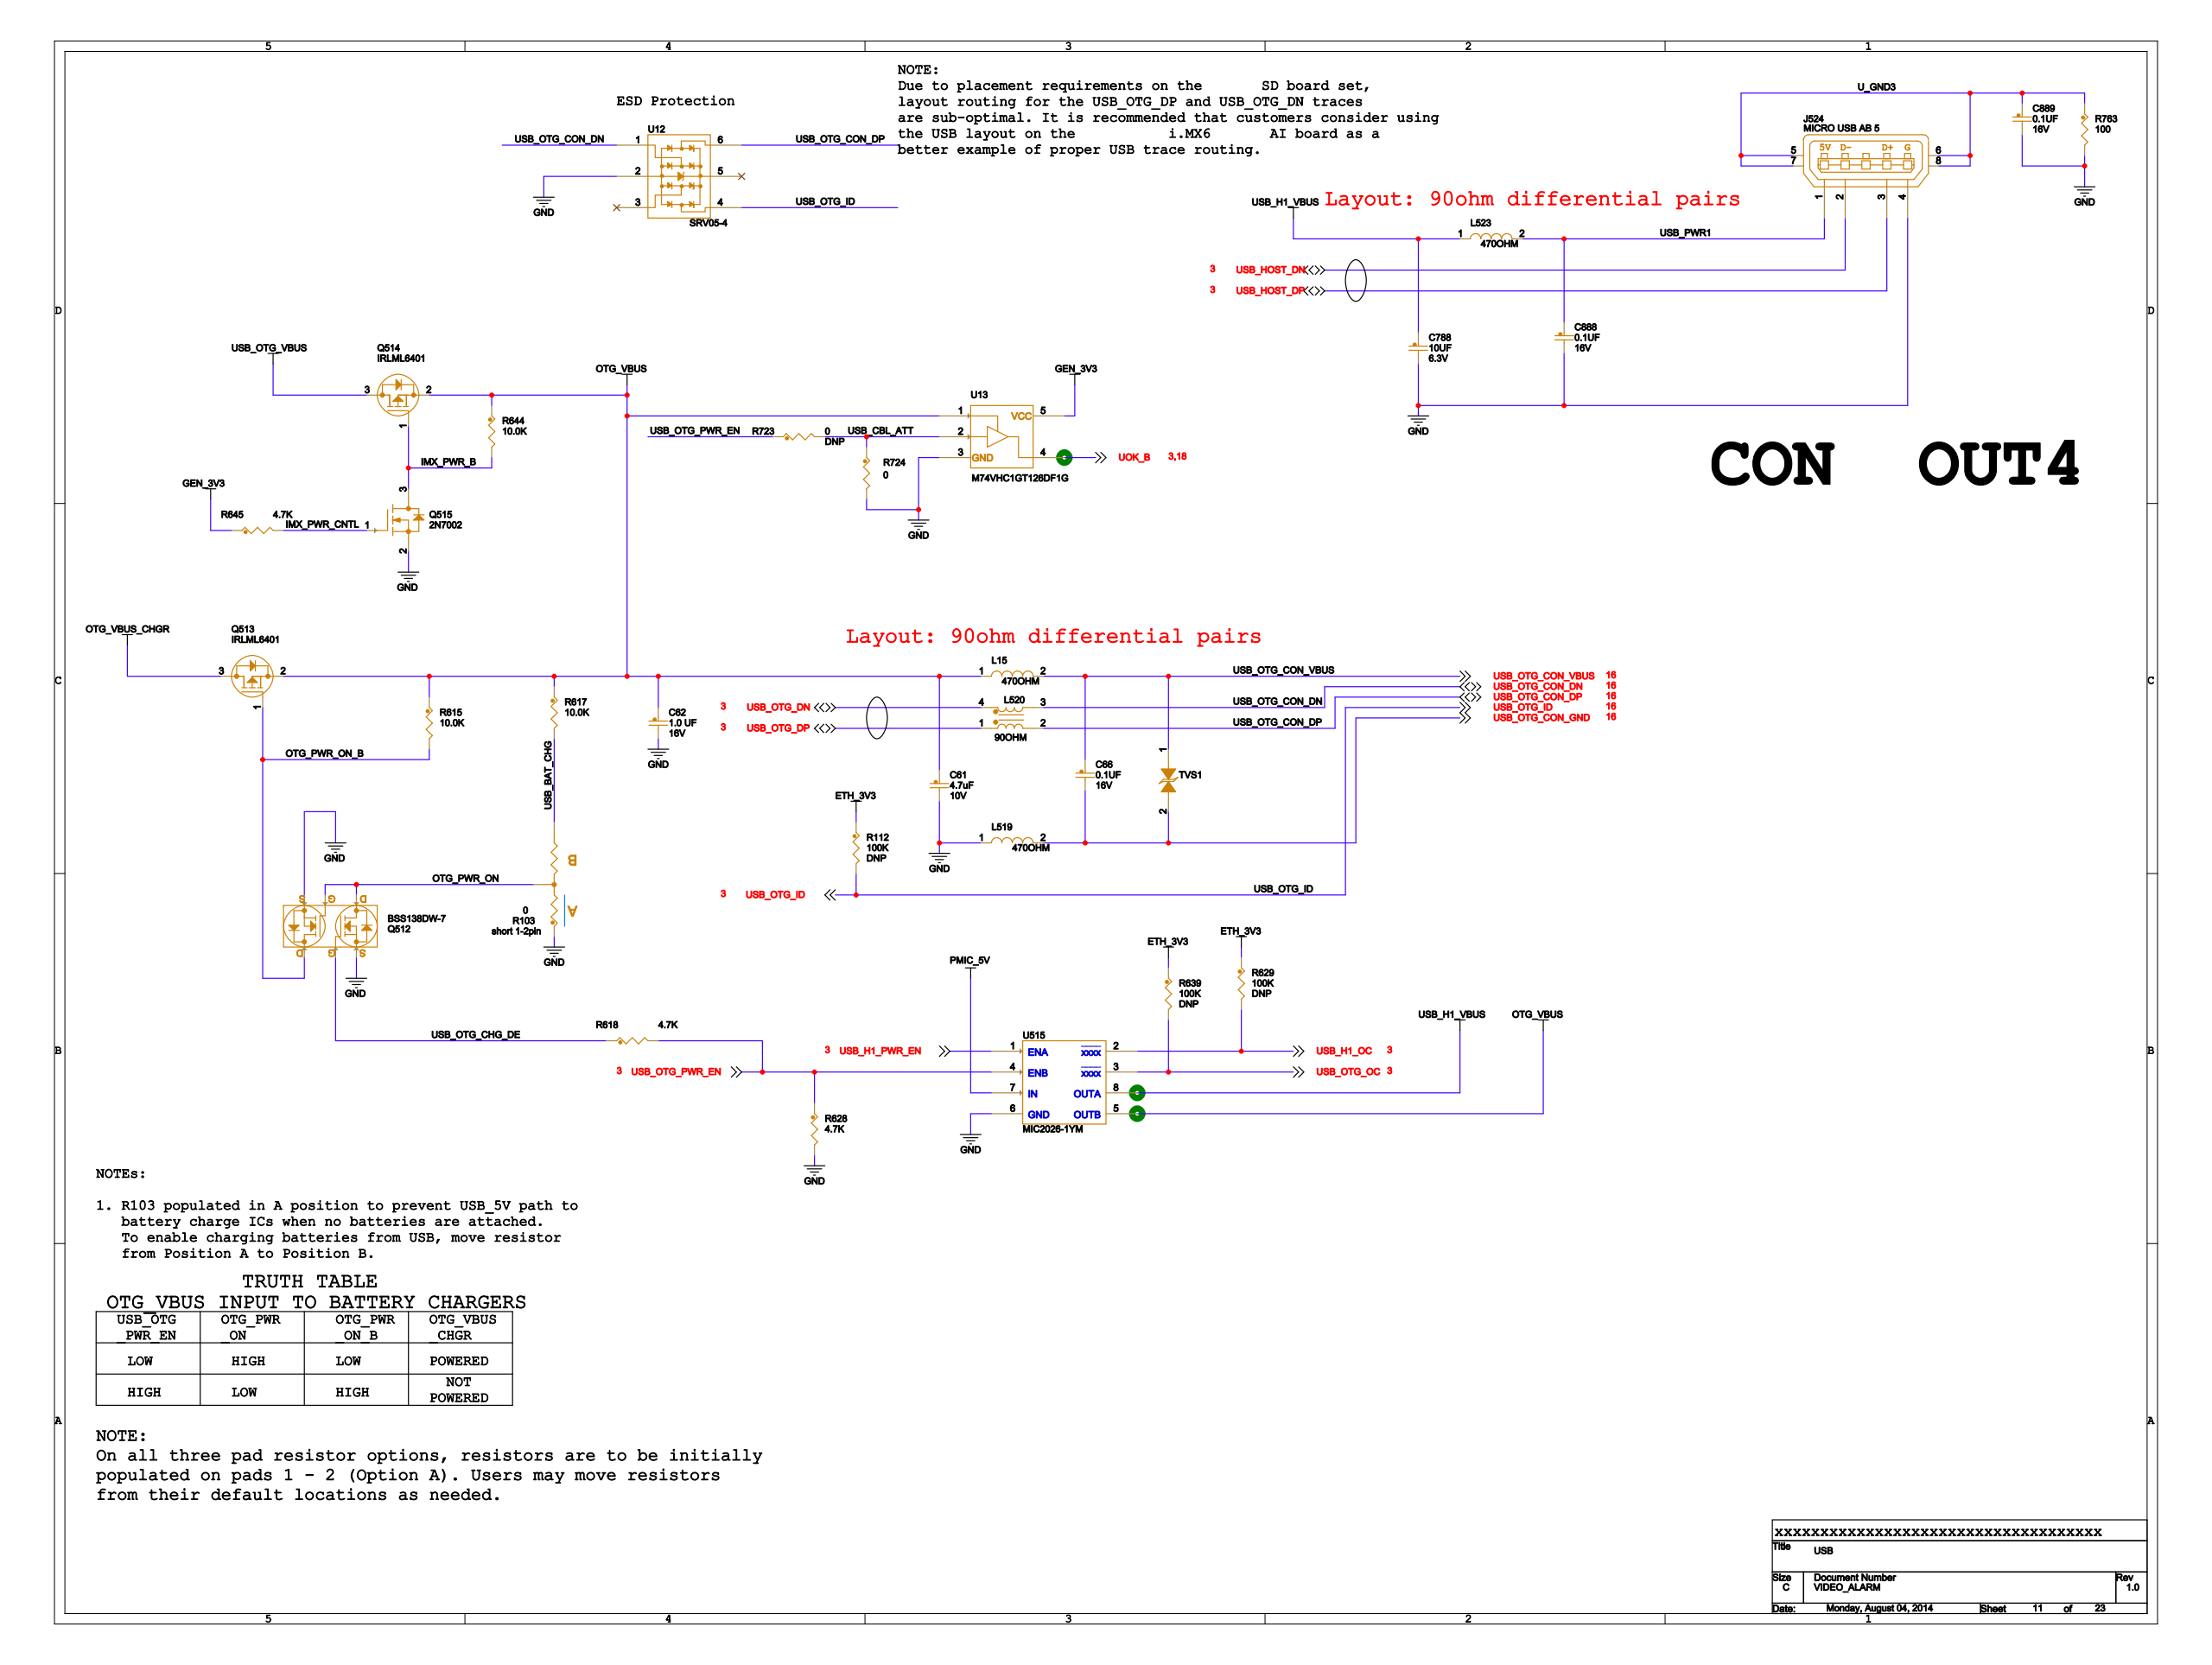Circuit board | Cadence Allegro | 994 parts | 728 nets | one sheet of the schematic
Parts on this sheet (reference | value | footprint):
C61 | 4.7uF | 0603_CC
C62 | 1.0 UF | 0603_CC
C66 | 0.1UF | 0603_CC
C788 | 10UF | 0603_CC
C888 | 0.1UF | 0603_CC
C889 | 0.1UF | 0603_CC
J524 | MICRO USB AB 5 | USB_A-RECEPT-R_A-DIP_1
L15 | 470OHM | 0603_CC
L519 | 470OHM | 0603_CC
L520 | 90OHM | IND4_CHOKE_0805
L523 | 470OHM | 0603_CC
Q512 | BSS138DW-7 | SC70-6
Q513 | IRLML6401 | SOT-23
Q514 | IRLML6401 | SOT-23
Q515 | 2N7002 | SOT23
R103 | 0 | R603-X2
R112 | 100K | 0603_CC
R615 | 10.0K | 0603_CC
R617 | 10.0K | 0603_CC
R618 | 4.7K | 0603_CC
R628 | 4.7K | 0603_CC
R629 | 100K | 0603_CC
R639 | 100K | 0603_CC
R644 | 10.0K | 0603_CC
R645 | 4.7K | 0603_CC
R723 | 0 | 0603_CC
R724 | 0 | 0603_CC
R763 | 100 | 0603_CC
TVS1 | ESD9B3.3ST5G | SOD-923_NP
U12 | SRV05-4 | SOT23_S6
U13 | M74VHC1GT126DF1G | SOT353
U515 | MIC2026-1YM | SO8
Nets of these parts (net: part-pin ...):
GND: C61-2 C62-2 C788-2 C888-2 C889-2 J524-4 L519-1 Q512-1 Q512-4 Q515-2 R103-1 R628-2 R724-2 R763-2 U12-2 U13-3 U515-6
GEN_3V3: R645-1 U13-5
PMIC_5V: U515-7
USB_OTG_CON_VBUS: C66-1 L15-2 TVS1-1
USB_OTG_CON_DN: L520-3 U12-1
USB_OTG_ID: R112-2 U12-4
USB_OTG_CON_DP: L520-2 U12-6
USB_OTG_CON_GND: C66-2 L519-2 TVS1-2
ETH_3V3: R112-1 R629-1 R639-1
USB_OTG_OC: R639-2 U515-3
USB_H1_OC: R629-2 U515-2
U_GND3: C889-1 J524-5 J524-6 J524-7 J524-8 R763-1
USB_CBL_ATT: R723-2 R724-1 U13-2
USB_OTG_PWR_EN: R618-2 R628-1 R723-1 U515-4
OTG_VBUS_CHGR: Q513-3
OTG_VBUS: C61-1 C62-1 L15-1 Q513-2 Q514-2 R615-1 R617-1 R644-1 U13-1 U515-5
IMX_PWR_B: Q514-1 Q515-3 R644-2
USB_BAT_CHG: R103-3 R617-2
OTG_PWR_ON_B: Q512-6 Q513-1 R615-2
UOK_B: U13-4
USB_PWR1: C888-1 J524-1 L523-2
USB_H1_PWR_EN: U515-1
USB_H1_VBUS: C788-1 L523-1 U515-8
USB_HOST_DN: J524-2
USB_HOST_DP: J524-3
USB_OTG_DN: L520-4
USB_OTG_DP: L520-1
USB_OTG_VBUS: Q514-3
IMX_PWR_CNTL: Q515-1 R645-2
USB_OTG_CHG_DE: Q512-5 R618-1
OTG_PWR_ON: Q512-2 Q512-3 R103-2